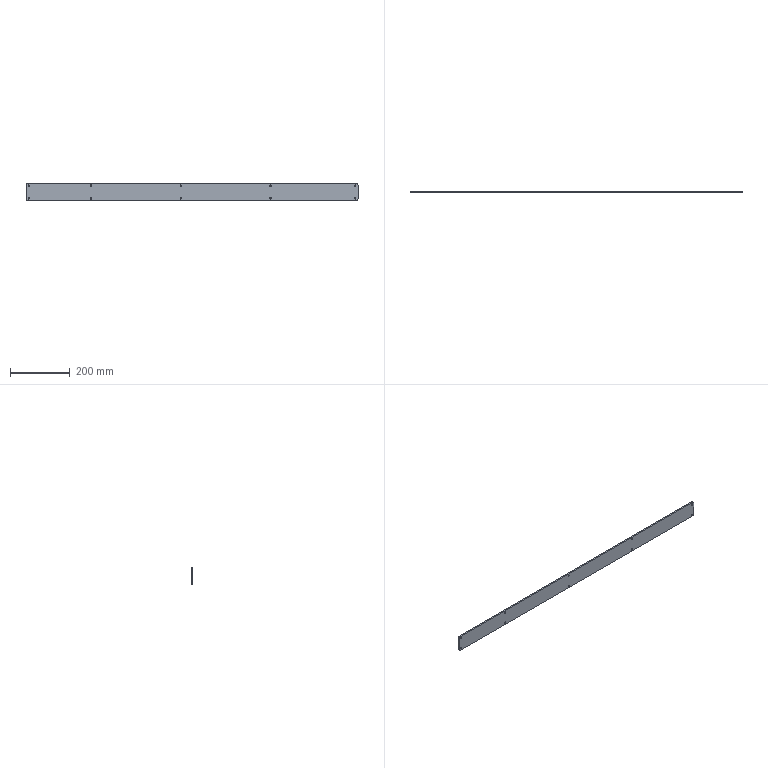Part | STEP file | DCV-000-036-2300L | 1 solid | 34 faces | box 1110 x 5 x 56 mm | volume 309711 mm3 | cylinder 28 | plane 6 | commonest cylinder face diameters 5 x20 10 x8